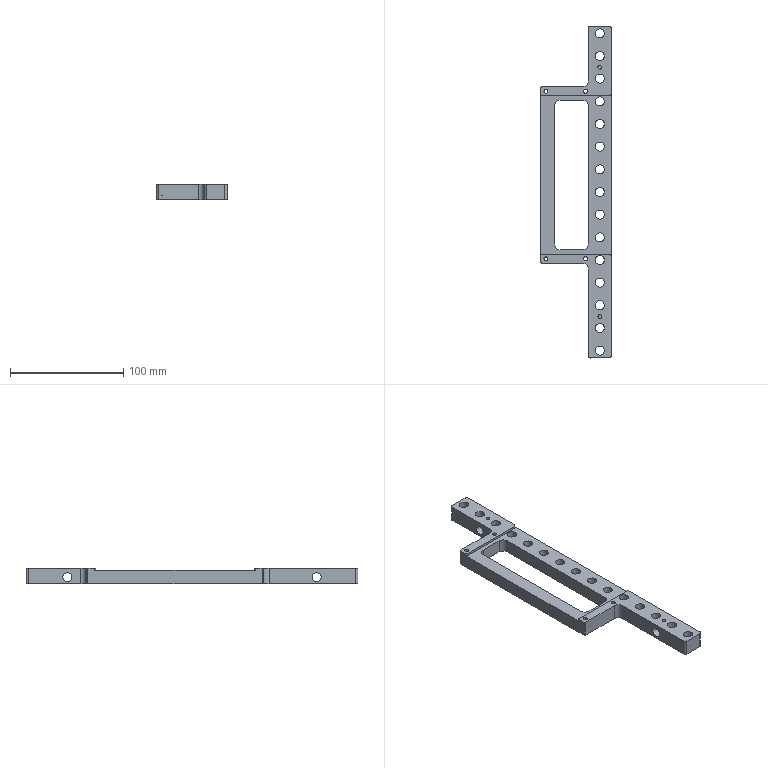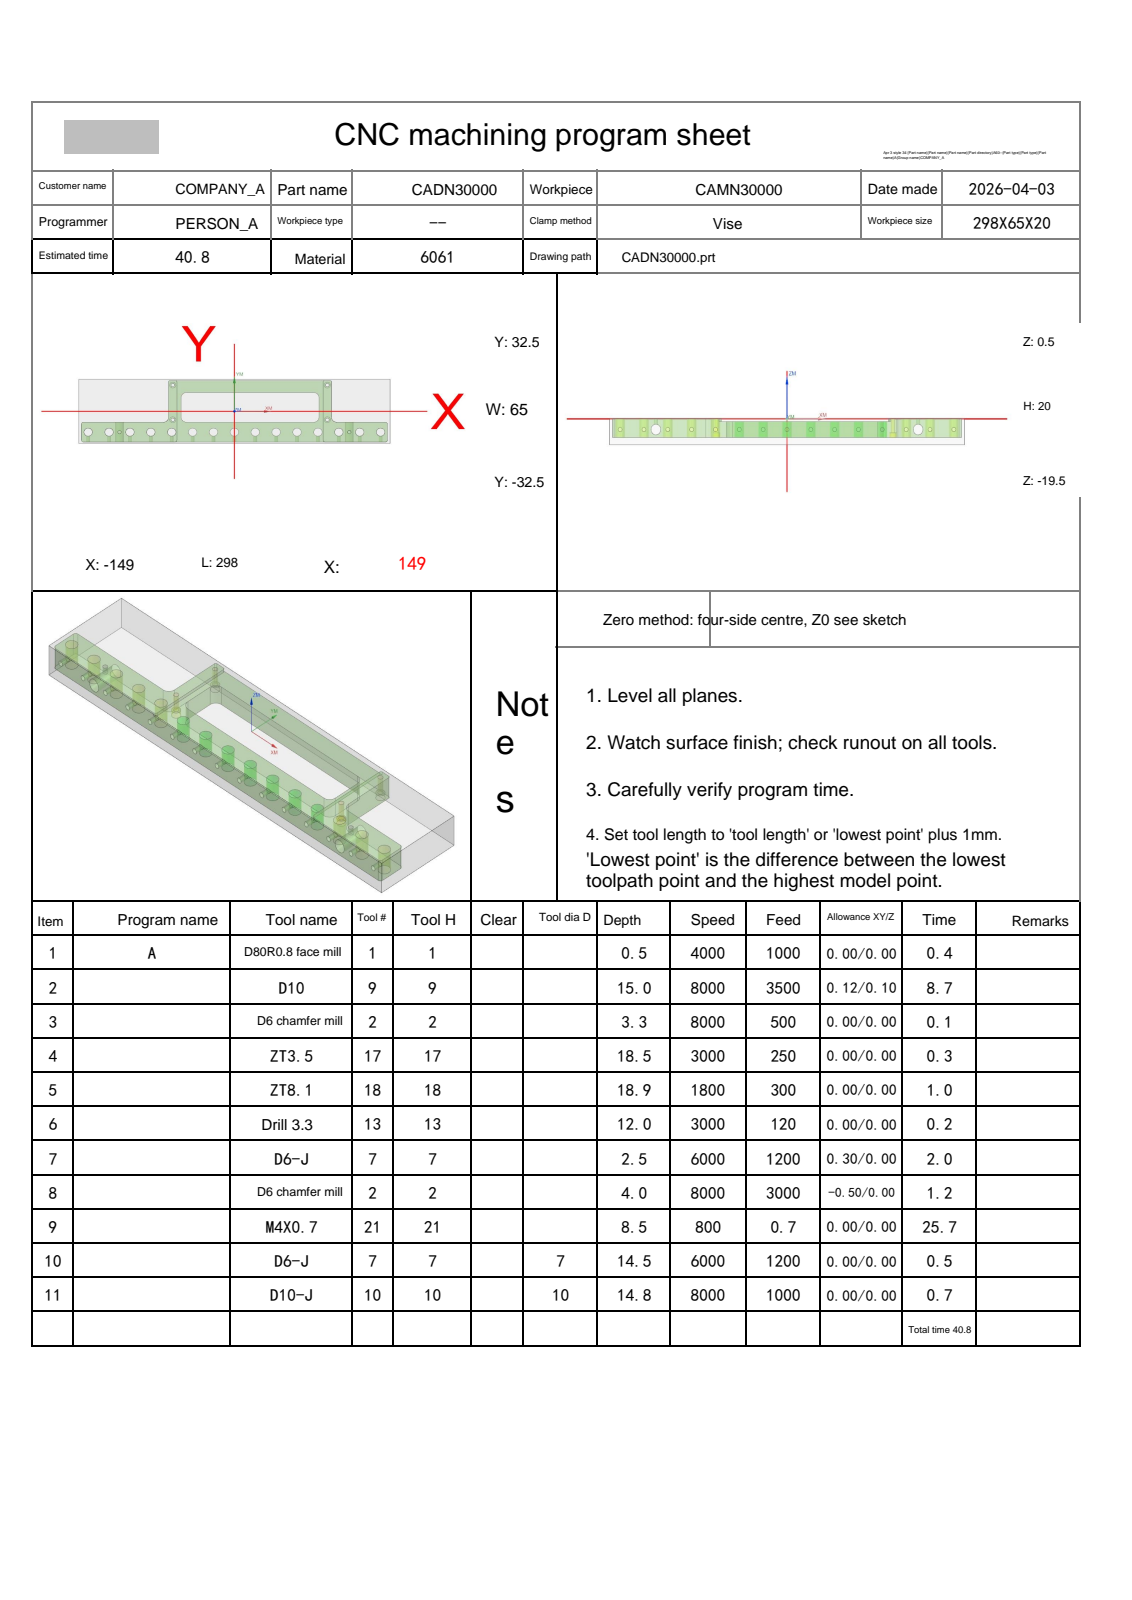NC program | NX | posted by the shop | part box 62 x 293 x 14 mm
Lines 36 to 825 of 5964:
N2 T09 M06
(D10  D=10. R=0. H=09 ce=0.12 di=0.10)
G00 G90 G54 X88.366 Y43.445 M03 S8000
G43 H09 Z20.
M08
Z-12.5
G01 X88.382 Y43.346 Z-13.125 F3500.
X88.398 Y43.248 Z-13.372
X88.414 Y43.149 Z-13.554
X88.43 Y43.05 Z-13.7
X88.446 Y42.951 Z-13.823
X88.462 Y42.853 Z-13.928
X88.477 Y42.754 Z-14.02
X88.493 Y42.655 Z-14.1
X88.509 Y42.557 Z-14.17
X88.525 Y42.458 Z-14.232
X88.541 Y42.359 Z-14.286
X88.557 Y42.26 Z-14.333
X88.573 Y42.162 Z-14.374
X88.589 Y42.063 Z-14.408
X88.605 Y41.964 Z-14.436
X88.621 Y41.866 Z-14.46
X88.637 Y41.767 Z-14.477
X88.653 Y41.668 Z-14.49
X88.669 Y41.569 Z-14.497
X88.685 Y41.471 Z-14.5
X89.019 Y39.395
G03 X89.346 Y39.001 I.503 J.084
X93.178 Y38.428 I3.876 J12.834
X101.853 Y38.295 I8.675 J282.345
X103.591 Y38.3 I0.0 J282.478
G01 X147.341 Y38.279
G02 X153.274 Y34.249 I-.2 J-6.677
X154.598 Y28.401 I-14.951 J-6.46
X154.816 Y19.492 I-182.174 J-8.909
X154.799 Y16.995 I-182.392 J0.0
G01 X154.774 Y-30.916
G02 X150.636 Y-36.838 I-6.704 J.279
X144.785 Y-38.108 I-6.434 J15.52
X136.71 Y-38.306 I-8.075 J164.923
X135.059 Y-38.297 I0.0 J165.121
G01 X-147.297 Y-38.281
G02 X-153.302 Y-34.188 I.172 J6.703
X-154.592 Y-28.479 I14.987 J6.387
X-154.808 Y-20.334 I153.312 J8.145
X-154.797 Y-18.544 I153.528 J0.0
G01 X-154.781 Y30.807
G02 X-150.823 Y36.737 I6.655 J-.155
X-145.06 Y38.085 I6.436 J-14.522
X-136.504 Y38.313 I8.556 J-160.427
X-134.284 Y38.298 I0.0 J-160.655
G01 X86.835 Y38.28
G03 X95.108 Y37.694 I15.608 J161.802
X104.71 Y37.6 I10.76 J603.908
G01 X145.579 Y37.575
G02 X152.002 Y33.432 I-.437 J-7.727
X153.764 Y27.207 I-14.23 J-7.39
X154.1 Y18.985 I-100.433 J-8.222
X154.092 Y17.697 I-100.769 J0.0
G01 X154.082 Y-28.92
G02 X149.838 Y-35.56 I-7.748 J.276
X143.669 Y-37.269 I-7.335 J14.483
X135.419 Y-37.6 I-8.25 J102.539
X134.088 Y-37.592 I0.0 J102.871
G01 X-145.579 Y-37.574
G02 X-152.028 Y-33.382 I.448 J7.745
X-153.755 Y-27.288 I14.212 J7.317
X-154.109 Y-18.528 I108.053 J8.761
X-154.094 Y-16.728 I108.408 J0.0
G01 X-154.074 Y29.079
G02 X-149.934 Y35.499 I7.732 J-.442
X-143.711 Y37.263 I7.389 J-14.205
X-135.007 Y37.608 I8.704 J-109.463
X-133.22 Y37.594 I0.0 J-109.809
G01 X85.239 Y37.58
X94.165 Y37.052
G03 X105.254 Y36.9 I11.089 J403.419
G01 X105.971
X143.761 Y36.876
G02 X151.325 Y31.864 I-.379 J-8.786
X153.058 Y25.265 I-16.654 J-7.9
X153.403 Y16.333 I-115.465 J-8.932
X153.392 Y14.774 I-115.81 J0.0
G01 X153.374 Y-27.286
G02 X149.06 Y-34.446 I-8.646 J.33
X147.589 Y-35.415 I-7.188 J9.308
X142.704 Y-36.512 I-6.118 J15.825
X133.383 Y-36.901 I-9.321 J111.513
X131.796 Y-36.889 I0.0 J111.902
G01 X120.456 Y-36.934
X-143.784 Y-36.911
G02 X-151.347 Y-31.833 I.451 J8.842
X-153.091 Y-24.951 I17.19 J8.019
X-153.407 Y-15.747 I133.706 J9.204
X-153.395 Y-13.899 I134.023 J0.0
G01 X-153.376 Y27.251
G02 X-148.452 Y34.777 I8.767 J-.362
X-141.728 Y36.561 I7.972 J-16.484
X-132.791 Y36.903 I8.937 J-116.735
X-131.237 Y36.892 I0.0 J-117.076
G01 X84.353 Y36.897
G03 X95.942 Y36.315 I40.76 J695.754
X108.127 Y36.2 I12.186 J649.067
G01 X108.771 Y36.201
X142.011 Y36.178
G02 X150.616 Y30.523 I-.151 J-9.604
X152.349 Y23.626 I-18.426 J-8.297
X152.71 Y13.834 I-132.729 J-9.792
X152.694 Y11.805 I-133.09 J0.0
G01 X152.678 Y-25.494
G02 X151.497 Y-30.094 I-10.288 J.19
G01 X151.441 Y-30.584
X150.915 Y-32.089
X150.067 Y-33.439
X148.939 Y-34.567
X147.589 Y-35.415
X146.084 Y-35.941
X144.499 Y-36.12
G03 X140.656 Y-36.111 I-3.843 J-851.591
X127.053 Y-36.22 I0.0 J-851.599
G01 X-141.947 Y-36.214
G03 X-144.09 Y-36.115 I-2.143 J-23.31
X-144.551 Y-36.12 I0.0 J-23.409
G02 X-149.503 Y-34.065 I.184 J7.44
X-151.481 Y-30.398 I5.506 J5.336
X-152.651 Y-18.3 I61.95 J12.098
G01 Y-18.008
X-152.698 Y-6.669
X-152.676 Y25.521
G02 X-147.023 Y34.115 I9.603 J-.161
X-140.126 Y35.849 I8.299 J-18.429
X-130.543 Y36.206 I9.583 J-128.416
X-128.726 Y36.193 I0.0 J-128.773
G01 X83.203 Y36.19
G03 X89.056 Y36.095 I5.853 J180.683
X92.056 Y36.12 I0.0 J180.778
G01 X95.389 Y35.757
G03 X105.774 Y35.49 I10.384 J201.862
X108.004 Y35.502 I0.0 J202.129
G01 X140.401 Y35.479
X140.483
G02 X149.893 Y29.319 I0.0 J-10.267
X151.663 Y21.93 I-20.181 J-8.74
X152.006 Y11.971 I-144.341 J-9.96
X151.993 Y10.039 I-144.684 J0.0
G01 X151.974 Y-23.971
G02 X151.62 Y-26.711 I-15.929 J.665
X151.642 Y-27.66 I-20.474 J-.95
X151.494 Y-30.114 I-20.497 J0.0
G03 X151.642 Y-27.66 I-20.349 J2.454
X151.62 Y-26.711 I-20.497 J0.0
G01 X151.6 Y-12.748
G02 X151.415 Y-3.423 I235.684 J9.325
X151.438 Y-.139 I235.869 J0.0
G03 X151.462 Y4.984 I-546.305 J5.122
X151.294 Y18.53 I-546.329 J0.0
X150.167 Y26.549 I-32.804 J-.521
X146.046 Y32.653 I-10.914 J-2.926
X140.146 Y34.657 I-6.784 J-10.285
X132.863 Y34.949 I-7.283 J-90.673
X131.335 Y34.936 I0.0 J-90.965
G01 X102.307 Y34.973
X101.985
G02 X95.085 Y35.29 I0.0 J75.218
G03 X92.93 Y36.05 I-3.605 J-6.789
G02 X95.408 Y35.119 I-1.66 J-8.189
G03 X99.93 Y34.419 I4.81 J16.098
X110.881 Y34.22 I10.952 J302.329
X114.371 Y34.241 I0.0 J302.527
G01 X134.521 Y34.207
G02 X135.037 Y34.211 I.516 J-33.098
X141.204 Y33.631 I0.0 J-33.102
X148.834 Y27.019 I-2.414 J-10.494
X150.438 Y19.518 I-22.691 J-8.776
X150.751 Y8.948 I-178.642 J-10.57
X150.735 Y6.575 I-178.954 J0.0
G03 X150.715 Y1.57 I622.281 J-5.004
X150.817 Y-9.709 I622.301 J0.0
G01 X151.441 Y-11.416
X151.62 Y-13.001
X151.441 Y-11.416
G02 X150.638 Y-9.193 I113.202 J42.201
X150.219 Y-4.29 I28.533 J4.903
X150.222 Y-3.904 I28.951 J0.0
G01 X150.114 Y13.934
Y14.014
G03 X149.36 Y22.851 I-52.142 J0.0
X146.54 Y29.26 I-14.062 J-2.361
X139.925 Y33.001 I-8.623 J-7.531
X132.902 Y33.633 I-7.023 J-38.658
G01 X132.683
X124.283 Y33.68
X104.973 Y33.716
G02 X104.369 Y33.713 I-.604 J51.363
X97.249 Y34.209 I0.0 J51.367
X96.075 Y34.556 I.273 J3.085
G01 X95.045 Y35.296
G03 X96.608 Y34.192 I15.019 J19.605
X100.851 Y33.274 I4.843 J12.127
X110.41 Y32.967 I9.559 J148.731
X112.555 Y32.983 I0.0 J149.038
G02 X118.974 Y33.004 I6.419 J-970.298
X133.331 Y32.898 I0.0 J-970.319
X140.12 Y32.046 I-.082 J-28.13
X147.592 Y25.181 I-3.085 J-10.857
X149.192 Y17.397 I-24.032 J-8.997
X149.491 Y6.608 I-195.087 J-10.789
X149.476 Y4.197 I-195.386 J0.0
G03 X149.457 Y1.765 I161.418 J-2.432
X149.674 Y-6.599 I161.436 J0.0
X149.978 Y-8.456 I6.431 J.1
G01 X150.849 Y-9.805
X149.832 Y-8.234
G02 X149.113 Y-4.484 I10.992 J4.053
X148.898 Y4.66 I194.486 J9.144
X148.908 Y6.663 I194.701 J0.0
G03 X148.918 Y8.24 I-122.885 J1.576
X148.514 Y18.202 I-122.895 J0.0
X146.65 Y25.415 I-20.899 J-1.553
X139.073 Y31.428 I-10.294 J-5.19
X131.515 Y32.335 I-7.651 J-31.802
X117.611 Y32.443 I-13.904 J-894.391
X111.855 Y32.425 I0.0 J-894.499
G02 X110.047 Y32.411 I-1.808 J119.155
X100.806 Y32.77 I0.0 J119.169
X96.864 Y33.717 I.705 J11.616
G01 X96.105 Y34.522
G03 X97.606 Y33.177 I4.301 J3.287
X102.234 Y32.076 I5.428 J12.533
X111.984 Y31.711 I9.75 J130.033
X113.888 Y31.724 I0.0 J130.398
G02 X118.722 Y31.743 I4.835 J-621.9
X131.51 Y31.612 I0.0 J-621.919
X138.767 Y30.588 I-.253 J-28.031
X146.42 Y23.228 I-3.501 J-11.299
X147.955 Y15.21 I-26.155 J-9.164
X148.243 Y3.184 I-251.31 J-12.026
X148.237 Y1.51 I-251.597 J0.0
G03 X148.231 Y.722 I51.384 J-.788
X148.671 Y-5.984 I51.39 J0.0
X149.155 Y-7.649 I5.264 J.628
G01 X149.996 Y-8.491
G02 X148.846 Y-7.204 I3.733 J4.496
X147.927 Y-3.139 I10.836 J4.586
X147.624 Y6.59 I156.211 J9.729
X147.629 Y7.812 I156.514 J0.0
G03 X147.632 Y8.505 I-76.835 J.694
X147.025 Y18.146 I-76.838 J0.0
X144.602 Y25.099 I-17.244 J-2.11
X137.389 Y30.105 I-10.102 J-6.854
X129.836 Y31.055 I-7.901 J-32.347
X115.29 Y31.184 I-14.545 J-815.993
X111.734 Y31.176 I0.0 J-816.123
G02 X110.666 Y31.17 I-1.068 J86.796
X101.749 Y31.629 I0.0 J86.803
X97.643 Y32.785 I1.053 J11.616
X96.907 Y33.658 I.902 J1.508
G03 X98.84 Y31.921 I3.016 J1.412
X104.269 Y30.787 I6.391 J17.048
X114.274 Y30.454 I10.005 J149.964
X116.058 Y30.465 I0.0 J150.297
G02 X119.471 Y30.483 I3.413 J-322.485
X130.533 Y30.293 I0.0 J-322.503
X137.685 Y29.076 I-.673 J-25.582
X145.234 Y21.349 I-4.145 J-11.601
X146.71 Y13.178 I-28.114 J-9.296
X147.023 Y1.232 I-328.91 J-14.604
G01 Y1.221
G03 X147.651 Y-5.269 I33.863 J0.0
X148.346 Y-7.049 I4.852 J.868
G02 X149.137 Y-7.631 I-1.71 J-3.154
G03 X148.278 Y-7.009 I-2.761 J-2.91
G02 X147.095 Y-4.269 I4.712 J3.659
X146.455 Y2.855 I39.504 J7.142
G03 X146.05 Y14.004 I-189.773 J-1.315
X144.364 Y21.557 I-24.465 J-1.494
X136.045 Y28.719 I-11.47 J-4.91
X128.016 Y29.785 I-8.372 J-32.301
X111.675 Y29.94 I-16.342 J-860.498
G01 X111.555
G02 X111.071 Y29.938 I-.485 J65.235
X102.171 Y30.548 I0.0 J65.237
X98.111 Y31.915 I1.389 J10.837
X97.57 Y32.535 I.443 J.933
G01 X97.285 Y33.017
X97.776 Y32.084
G03 X100.474 Y30.482 I4.167 J3.943
X107.281 Y29.423 I7.662 J26.845
X119.233 Y29.178 I11.952 J291.171
X121.734 Y29.188 I0.0 J291.416
G02 X122.976 Y29.197 I1.242 J-85.634
X131.937 Y28.727 I0.0 J-85.643
X138.915 Y26.392 I-1.675 J-16.599
X144.127 Y19.274 I-7.391 J-10.878
X145.483 Y10.935 I-31.496 J-9.401
G01 X145.872 Y.528
G03 X146.819 Y-5.251 I21.767 J.6
X147.512 Y-6.54 I3.225 J.903
G01 X148.36 Y-7.069
G02 X147.297 Y-6.38 I4.276 J7.761
X145.935 Y-3.318 I5.374 J4.224
X145.2 Y3.82 I39.475 J7.671
G03 X144.65 Y13.644 I-124.937 J-2.076
X142.528 Y21.148 I-20.959 J-1.872
X134.503 Y27.413 I-11.287 J-6.187
X126.616 Y28.503 I-8.482 J-32.308
X112.138 Y28.701 I-17.158 J-725.643
G01 X111.952 Y28.7
G02 X102.748 Y29.433 I0.0 J58.195
X98.529 Y31.006 I1.637 J10.831
X97.641 Y32.322 I.975 J1.616
G03 X99.338 Y30.169 I3.06 J.665
X104.602 Y28.568 I6.827 J12.992
X114.706 Y27.967 I10.105 J84.66
X115.396 Y27.969 I0.0 J85.261
G02 X116.713 Y27.973 I1.317 J-222.994
X127.905 Y27.692 I0.0 J-222.998
X135.413 Y26.139 I-1.033 J-23.912
X142.645 Y18.319 I-5.068 J-11.943
X144.161 Y10.296 I-28.53 J-9.546
G03 X144.714 Y.645 I830.765 J42.782
X145.872 Y-4.861 I18.699 J1.055
X146.818 Y-6.305 I3.644 J1.357
G01 X147.589 Y-6.585
G02 X146.428 Y-6.031 I.536 J2.62
X144.864 Y-2.877 I5.344 J4.614
X143.961 Y4.118 I35.441 J8.13
G03 X143.215 Y13.299 I-97.979 J-3.343
X140.689 Y20.597 I-18.635 J-2.364
X133.045 Y26.099 I-11.066 J-7.312
X124.745 Y27.245 I-8.833 J-33.348
X112.041 Y27.482 I-24.212 J-955.997
G02 X103.123 Y28.343 I.362 J50.403
X98.746 Y30.166 I1.862 J10.635
X98.009 Y31.039 I1.125 J1.698
G03 X97.871 Y31.629 I-3.67 J-.546
G01 X98.094 Y30.732
G03 X100.256 Y28.843 I4.068 J2.475
X106.133 Y27.263 I7.651 J16.741
X116.047 Y26.716 I10.002 J91.146
G01 X116.507 Y26.717
G02 X127.227 Y26.341 I0.0 J-153.093
X134.667 Y24.506 I-1.388 J-21.629
X141.382 Y16.783 I-5.915 J-11.924
X142.903 Y8.971 I-29.365 J-9.77
G03 X143.594 Y.576 I240.014 J15.551
X145.04 Y-4.796 I16.033 J1.434
X145.972 Y-6.016 I3.29 J1.547
G01 X146.843 Y-6.324
G02 X145.634 Y-5.82 I.857 J3.754
X143.891 Y-2.823 I4.609 J4.687
X142.745 Y4.032 I30.142 J8.561
G03 X141.834 Y12.491 I-87.453 J-5.136
X138.997 Y19.743 I-17.642 J-2.721
X131.316 Y24.88 I-11.053 J-8.216
X123.079 Y25.984 I-8.918 J-35.257
G01 X111.682 Y26.287
G02 X103.065 Y27.349 I.868 J42.508
X98.814 Y29.391 I2.175 J9.973
X98.081 Y30.361 I1.697 J2.045
G01 X98.014 Y30.988
Y30.959
G03 X99.096 Y28.802 I2.691 J0.0
X103.573 Y26.684 I6.783 J8.544
X112.329 Y25.598 I9.776 J42.992
G02 X123.982 Y25.208 I-19.123 J-744.989
X131.942 Y23.755 I-.999 J-28.02
X140.137 Y15.244 I-4.72 J-12.745
X141.73 Y7.159 I-32.559 J-10.614
G03 X142.715 Y-.663 I77.16 J5.741
X144.483 Y-5.136 I11.409 J1.925
X145.455 Y-5.988 I1.877 J1.162
G01 X146.084 Y-6.059
X146.011 Y-6.06
G02 X144.252 Y-5.149 I0.0 J2.153
X142.364 Y-.999 I8.217 J6.244
X141.232 Y6.584 I57.767 J12.494
G03 X139.701 Y14.399 I-35.945 J-2.987
X130.284 Y23.469 I-13.123 J-4.201
X122.067 Y24.701 I-9.157 J-33.072
G02 X110.6 Y25.158 I19.419 J630.622
X102.53 Y26.517 I1.478 J33.436
X98.725 Y28.725 I2.577 J8.822
X98.12 Y29.687 I1.583 J1.667
G01 X98.083 Y30.347
G03 X98.168 Y29.364 I14.767 J.79
X100.134 Y27.166 I4.262 J1.835
X105.962 Y25.101 I8.197 J13.87
X115.37 Y24.252 I10.709 J66.197
G02 X125.068 Y23.707 I-1.974 J-121.495
X132.549 Y21.531 I-1.839 J-20.268
X138.866 Y13.836 I-6.928 J-12.128
X140.484 Y6.465 I-33.385 J-11.191
G03 X141.701 Y-.842 I61.107 J6.421
X143.669 Y-5.099 I10.717 J2.371
X144.654 Y-5.897 I2.035 J1.506
G01 X145.419 Y-5.984
X145.369
G02 X144.155 Y-5.706 I0.0 J2.793
X142.021 Y-2.925 I3.608 J4.978
X140.39 Y3.382 I23.343 J9.4
G03 X139.048 Y10.999 I-81.989 J-10.517
X135.378 Y18.232 I-16.077 J-3.61
X127.564 Y22.542 I-10.936 J-10.589
X119.094 Y23.533 I-9.544 J-44.899
G02 X108.374 Y24.217 I3.44 J138.21
X101.314 Y26.045 I2.196 J23.024
X98.271 Y28.572 I2.654 J6.293
X98.096 Y29.366 I1.715 J.795
X98.12 Y29.667 I1.891 J0.0
G03 X98.096 Y29.303 I2.804 J-.364
X99.032 Y27.201 I2.828 J0.0
X103.562 Y24.639 I7.36 J7.726
X112.106 Y23.213 I10.481 J36.501
G02 X122.267 Y22.594 I-29.996 J-576.291
X130.074 Y20.783 I-1.629 J-24.748
X137.528 Y12.678 I-5.848 J-12.858
X139.253 Y5.832 I-33.62 J-12.112
G03 X140.759 Y-1.21 I50.777 J7.178
X142.954 Y-5.21 I9.762 J2.755
X143.952 Y-5.88 I1.67 J1.408
G01 X144.641 Y-5.896
G02 X144.423 Y-5.902 I-.217 J3.695
X143.625 Y-5.815 I0.0 J3.701
X141.476 Y-3.704 I2.251 J4.44
X139.496 Y1.797 I16.145 J8.919
G03 X137.981 Y9.094 I-243.44 J-46.732
X134.67 Y16.21 I-17.877 J-3.991
X126.887 Y21.078 I-11.38 J-9.539
X118.445 Y22.269 I-9.974 J-40.191
G02 X108.056 Y23.13 I4.617 J118.839
X101.213 Y25.139 I2.655 J21.704
X98.259 Y27.766 I2.949 J6.29
X98.097 Y28.541 I1.773 J.775
X98.12 Y28.841 I1.935 J0.0
G03 X98.1 Y28.491 I3.029 J-.35
X99.101 Y26.232 I3.05 J0.0
X103.703 Y23.559 I7.742 J8.029
X112.369 Y21.996 I11.043 J36.416
G02 X121.563 Y21.274 I-22.661 J-347.552
X129.307 Y19.212 I-1.996 J-23.071
X136.307 Y11.304 I-6.669 J-12.954
X138.166 Y4.633 I-38.729 J-14.393
G03 X140.063 Y-2.116 I35.832 J6.426
X142.566 Y-5.597 I7.696 J2.895
X143.142 Y-5.88 I1.12 J1.55
G01 X143.912
G02 X143.551 Y-5.904 I-.361 J2.767
X142.626 Y-5.746 I0.0 J2.791
X140.204 Y-3.204 I2.978 J5.262
X138.057 Y2.802 I20.622 J10.761
G03 X136.141 Y9.891 I-66.926 J-14.279
X130.826 Y17.313 I-14.562 J-4.815
X123.194 Y20.346 I-10.488 J-15.271
X114.484 Y21.269 I-13.237 J-83.368
G02 X105. Y22.671 I2.705 J51.082
X99.567 Y25.3 I3.252 J13.648
X98.12 Y27.26 I2.652 J3.472
G01 Y28.03
G03 X98.096 Y27.639 I3.18 J-.391
X99.091 Y25.319 I3.204 J0.0
X103.667 Y22.529 I7.998 J7.97
X112.105 Y20.823 I11.45 J34.92
G02 X121.288 Y19.889 I-17.64 J-219.055
X128.9 Y17.422 I-2.496 J-20.675
X135.118 Y9.955 I-7.96 J-12.95
X137.354 Y2.696 I-53.184 J-20.355
G03 X139.69 Y-3.371 I23.122 J5.421
X142.129 Y-5.854 I5.511 J2.974
G01 X143.098 Y-5.88
G02 X142.707 Y-5.905 I-.391 J3.107
X141.735 Y-5.75 I0.0 J3.132
X139.219 Y-3.251 I2.986 J5.523
X136.92 Y2.4 I20.319 J11.557
G03 X134.695 Y9.276 I-62.081 J-16.289
X124.462 Y18.463 I-14.265 J-5.596
X116.12 Y19.866 I-11.423 J-42.436
G02 X106.476 Y21.207 I5.236 J72.983
X100.297 Y23.765 I3.498 J17.193
X98.129 Y26.292 I3.137 J4.885
G01 X98.12 Y27.189
G03 X98.095 Y26.77 I3.546 J-.418
X98.325 Y25.51 I3.571 J0.0
X101.3 Y22.599 I6.329 J3.492
X108.299 Y20.211 I10.578 J19.547
X117.695 Y18.985 I21.976 J131.86
G02 X125.453 Y17.207 I-2.814 J-30.091
X133.761 Y9.095 I-5.827 J-14.276
X136.254 Y2.161 I-53.513 J-23.159
G03 X138.821 Y-3.607 I22.021 J6.344
X141.217 Y-5.859 I5.333 J3.272
G01 X142.234 Y-5.88
G02 X141.814 Y-5.905 I-.42 J3.542
X140.825 Y-5.765 I0.0 J3.567
X138.257 Y-3.377 I2.856 J5.646
X135.722 Y2.177 I20.576 J12.747
G03 X133.091 Y8.962 I-50.585 J-15.708
X123.027 Y17.252 I-14.225 J-7.015
X115.534 Y18.641 I-11.948 J-43.564
G02 X106.22 Y20.168 I6.572 J69.279
X100.099 Y22.926 I3.826 J16.66
X98.129 Y25.352 I3.333 J4.72
G01 X98.12 Y26.246
G03 X98.095 Y25.827 I3.524 J-.42
X98.37 Y24.456 I3.549 J0.0
X101.443 Y21.496 I6.68 J3.859
X108.432 Y19.041 I11.052 J20.288
X117.305 Y17.688 I28.911 J159.847
G02 X125.103 Y15.533 I-3.293 J-27.094
X132.585 Y7.92 I-7.15 J-14.51
X135.387 Y1.062 I-70.326 J-32.738
G03 X138.282 Y-4.272 I18.192 J6.42
X140.293 Y-5.872 I4.215 J3.235
G01 X141.254 Y-5.88
G02 X140.834 Y-5.905 I-.421 J3.608
X139.826 Y-5.762 I0.0 J3.633
X137.112 Y-3.281 I3.019 J6.028
X134.279 Y2.502 I24.682 J15.676
G03 X131.115 Y9.141 I-34.948 J-12.579
X121.698 Y16.035 I-13.843 J-9.031
X114.224 Y17.533 I-13.663 J-48.791
G02 X105.157 Y19.38 I6.48 J54.984
X99.603 Y22.348 I4.19 J14.52
X98.12 Y24.438 I3.107 J3.776
G01 Y25.278
G03 X98.095 Y24.858 I3.562 J-.42
X98.376 Y23.468 I3.587 J0.0
X101.533 Y20.408 I6.907 J3.968
X108.759 Y17.817 I11.722 J21.317
X117.264 Y16.317 I59.575 J312.943
G02 X124.985 Y13.682 I-3.835 J-23.867
X131.601 Y6.488 I-9.036 J-14.949
X134.582 Y.013 I-121.644 J-59.937
G03 X137.692 Y-4.777 I15.226 J6.479
X139.326 Y-5.88 I3.046 J2.752
G01 X140.306
G02 X139.849 Y-5.901 I-.457 J4.996
X138.986 Y-5.826 I0.0 J5.016
X136.364 Y-3.765 I2.269 J5.584
X133.383 Y1.437 I20.306 J15.094
G03 X130.045 Y7.823 I-41.358 J-17.552
X120.473 Y14.815 I-14.428 J-9.703
X114.264 Y16.234 I-14.035 J-47.113
G02 X105.512 Y18.161 I9.494 J63.952
X99.741 Y21.21 I4.497 J15.498
X98.12 Y23.457 I3.188 J4.008
G01 Y24.367
G03 X98.099 Y23.927 I4.573 J-.441
X98.241 Y22.792 I4.594 J0.0
X100.807 Y19.837 I6.228 J2.817
X107.451 Y16.978 I11.501 J17.576
X115.921 Y15.198 I35.314 J147.021
G02 X123.628 Y12.528 I-4.647 J-25.868
X130.362 Y5.627 I-9.324 J-15.836
X133.636 Y-.624 I-152.75 J-83.978
G03 X136.891 Y-5.04 I13.962 J6.885
X138.263 Y-5.88 I2.628 J2.751
G01 X139.313
G02 X138.863 Y-5.894 I-.451 J7.062
X137.942 Y-5.834 I0.0 J7.076
X135.202 Y-3.744 I2.301 J5.854
X131.973 Y1.47 I23.435 J18.121
G03 X128.004 Y7.857 I-31.953 J-15.433
X118.931 Y13.73 I-14.266 J-12.094
X111.222 Y15.545 I-21.812 J-75.339
G02 X103.054 Y18.036 I6.601 J36.287
X98.684 Y21.354 I4.451 J10.398
X98.12 Y22.448 I3.116 J2.3
G01 Y23.358
G03 X98.096 Y22.91 I4.108 J-.448
X98.3 Y21.626 I4.132 J0.0
X101.071 Y18.599 I6.7 J3.351
X108.041 Y15.653 I12.431 J19.699
X116.018 Y13.771 I127.377 J521.916
G02 X123.891 Y10.39 I-5.184 J-22.933
X129.822 Y3.699 I-12.791 J-17.311
G03 X133.244 Y-2.09 I154.932 J87.676
X136.474 Y-5.558 I10.038 J6.113
X137.161 Y-5.88 I1.724 J2.778
G01 X138.211
G02 X137.735 Y-5.898 I-.476 J6.203
X136.824 Y-5.831 I0.0 J6.222
X134.112 Y-3.858 I2.323 J6.041
X131.074 Y.519 I21.928 J18.464
G03 X126.948 Y6.625 I-36.698 J-20.351
X117.658 Y12.597 I-15.075 J-13.241
X109.827 Y14.633 I-31.473 J-104.937
G02 X102.189 Y17.398 I6.805 J30.726
X98.461 Y20.664 I4.516 J8.917
X98.12 Y21.423 I4.091 J2.293
G01 Y22.333
G03 X98.095 Y21.882 I4.112 J-.451
X98.306 Y20.58 I4.136 J0.0
X101.102 Y17.508 I6.861 J3.436
X107.983 Y14.484 I13.047 J20.348
G02 X115.969 Y12.337 I-234.723 J-888.76
X124.623 Y7.7 I-5.859 J-21.329
X129.478 Y1.665 I-19.975 J-21.038
G03 X133.182 Y-3.664 I39.914 J23.795
X135.946 Y-5.869 I6.171 J4.899
G01 X137.134 Y-5.88
G02 X136.636 Y-5.898 I-.497 J7.046
X135.677 Y-5.832 I0.0 J7.064
X132.803 Y-3.785 I2.438 J6.461
X129.192 Y1.109 I30.716 J26.447
G03 X123.985 Y7.325 I-25.063 J-15.706
X115.413 Y11.825 I-15.069 J-18.289
G01 X107.625 Y14.042
G02 X100.827 Y17.184 I6.441 J22.859
X98.14 Y20.282 I4.117 J6.285
G01 X98.12 Y21.297
G03 X98.096 Y20.847 I4.215 J-.449
X98.299 Y19.552 I4.239 J0.0
X101.132 Y16.403 I7.01 J3.458
X108.137 Y13.231 I13.961 J21.513
G02 X115.939 Y10.856 I-57.678 J-203.43
X127.159 Y2.583 I-7.357 J-21.722
G03 X131.228 Y-2.898 I160.351 J114.799
X134.608 Y-5.822 I8.554 J6.473
X135.52 Y-5.904 I.911 J5.011
X136.011 Y-5.88 I0.0 J5.093
G02 X135.529 Y-5.892 I-.482 J10.051
X134.495 Y-5.838 I0.0 J10.062
X131.564 Y-3.851 I2.414 J6.714
X127.715 Y.913 I35.884 J32.929
G03 X121.563 Y7.204 I-22.93 J-16.273
X113.467 Y11.011 I-16.229 J-23.996
G02 X105.58 Y13.58 I35.916 J123.685
X99.871 Y16.882 I6.273 J17.428
X98.12 Y19.324 I3.715 J4.514
G01 Y20.304
G03 X98.098 Y19.835 I4.946 J-.469
X98.244 Y18.637 I4.969 J0.0
X100.827 Y15.529 I6.716 J2.954
X107.463 Y12.236 I14.102 J20.082
G02 X115.111 Y9.652 I-83.62 J-260.121
X126.235 Y1.51 I-8.892 J-23.819
G03 X130.541 Y-3.66 I73.916 J57.196
X133.525 Y-5.875 I6.596 J5.768
G01 X134.82 Y-5.88
G02 X134.293 Y-5.894 I-.527 J10.053
X133.229 Y-5.838 I0.0 J10.067
X130.306 Y-3.957 I2.45 J7.021
X126.049 Y.849 I44.358 J43.576
G03 X113.516 Y9.565 I-21.289 J-17.243
G02 X105.826 Y12.296 I78.365 J232.911
X99.865 Y15.797 I6.778 J18.363
X98.12 Y18.255 I3.823 J4.563
G01 Y19.235
G03 X98.099 Y18.77 I5.269 J-.465
X98.23 Y17.603 I5.289 J0.0
X100.667 Y14.543 I6.651 J2.797
X107.088 Y11.143 I14.506 J19.629
G02 X114.584 Y8.347 I-84.386 J-237.711
X125.103 Y.732 I-10.846 J-26.053
G03 X129.592 Y-4.109 I57.581 J48.895
X132.156 Y-5.864 I6.417 J6.624
G01 X133.506 Y-5.88
G02 X133.046 Y-5.888 I-.46 J13.818
X131.916 Y-5.842 I0.0 J13.826
X128.861 Y-3.955 I2.548 J7.544
X124.347 Y.706 I63.767 J66.28
G03 X112.762 Y8.405 I-22.117 J-20.711
G02 X105.043 Y11.432 I60.174 J164.81
X99.544 Y15.008 I6.955 J16.715
X98.12 Y17.172 I3.792 J4.046
G01 Y18.152
G03 X98.095 Y17.672 I4.617 J-.48
X98.287 Y16.35 I4.642 J0.0
X100.936 Y13.204 I7.239 J3.407
X107.476 Y9.731 I16.213 J22.637
G02 X115.13 Y6.538 I-38.187 J-102.302
X124.282 Y-.342 I-14.78 J-29.186
G03 X128.793 Y-4.67 I36.361 J33.388
X130.859 Y-5.88 I4.451 J5.231
G01 X132.189
G02 X131.591 Y-5.905 I-.599 J7.198
X130.346 Y-5.797 I0.0 J7.223
X127.022 Y-3.69 I3.519 J9.228
X122.053 Y1.002 I488.449 J522.287
G03 X111.277 Y7.577 I-23.5 J-26.395
G02 X103.88 Y10.801 I32.684 J85.091
X99.112 Y14.372 I6.865 J14.135
X98.12 Y16.073 I3.87 J3.398
G01 Y17.053
G03 X98.095 Y16.573 I4.644 J-.48
X98.291 Y15.235 I4.669 J0.0
X100.919 Y12.07 I7.365 J3.441
X107.146 Y8.585 I16.946 J22.981
G02 X114.968 Y5.024 I-38.636 J-95.209
X123.551 Y-1.432 I-19.476 J-34.83
G03 X128.148 Y-5.273 I22.602 J22.377
X129.394 Y-5.88 I3.216 J5.02
G01 X130.794
G02 X130.324 Y-5.886 I-.47 J19.334
X129.054 Y-5.844 I0.0 J19.34
X125.861 Y-4.077 I2.652 J8.56
X120.492 Y.517 I243.93 J290.52
G03 X110.224 Y6.617 I-26.36 J-32.682
G02 X103.121 Y10.02 I26.775 J65.004
X98.819 Y13.624 I6.751 J12.43
X98.12 Y14.958 I3.865 J2.873
G01 Y15.938
G03 X98.095 Y15.457 I4.696 J-.482
X98.293 Y14.105 I4.72 J0.0
X101.003 Y10.834 I7.652 J3.581
X107.314 Y7.198 I18.892 J25.494
G02 X115.323 Y3.198 I-32.979 J-76.053
X122.894 Y-2.509 I-28.849 J-46.149
G03 X127.329 Y-5.69 I15.169 J16.467
G01 X127.836 Y-5.88
X129.376
G02 X128.689 Y-5.905 I-.687 J9.547
X127.312 Y-5.805 I0.0 J9.572
X123.792 Y-3.823 I3.748 J10.772
G03 X117.642 Y.945 I-126.999 J-157.46
X109.644 Y5.473 I-29.757 J-43.237
G02 X102.567 Y9.149 I25.975 J58.658
X98.612 Y12.787 I6.643 J11.19
X98.12 Y13.824 I4.236 J2.646
G01 Y14.874
G03 X98.099 Y14.377 I5.893 J-.496
X98.228 Y13.151 I5.914 J0.0
X100.649 Y9.942 I7.219 J2.928
X106.433 Y6.302 I18.166 J22.451
G02 X114.551 Y2.045 I-50.21 J-105.621
X122.009 Y-3.324 I-41.687 J-65.774
G03 X126.091 Y-5.865 I11.411 J13.784
G01 X127.789 Y-5.88
G02 X127.072 Y-5.904 I-.717 J10.738
X125.654 Y-5.81 I0.0 J10.762
X122.005 Y-3.879 I3.833 J11.657
G03 X115.198 Y.927 I-95.485 J-128.001
X106.828 Y5.479 I-51.487 J-84.71
G02 X100.504 Y9.484 I13.444 J28.224
X98.128 Y12.615 I5.046 J6.296
G01 X98.12 Y13.719
G03 X98.1 Y13.224 I6.103 J-.495
X98.222 Y12.006 I6.123 J0.0
X100.536 Y8.838 I7.244 J2.861
X106.463 Y4.945 I19.509 J23.244
G02 X115.382 Y-.087 I-49.016 J-97.304
G01 X121.763 Y-4.507
G03 X124.414 Y-5.88 I6.922 J10.115
G01 X126.164
G02 X125.386 Y-5.903 I-.777 J13.418
X123.902 Y-5.82 I0.0 J13.441
X120.27 Y-4.043 I3.719 J12.199
G03 X112.36 Y1.08 I-97.328 J-141.612
G02 X104.314 Y5.546 I476.229 J867.503
X99.239 Y9.579 I9.56 J17.238
X98.12 Y11.493 I4.374 J3.842
G01 Y12.543
G03 X98.1 Y12.048 I6.098 J-.495
X98.225 Y10.818 I6.118 J0.0
X100.546 Y7.603 I7.442 J2.93
X106.631 Y3.485 I21.42 J25.091
G02 X119.135 Y-4.118 I-70.784 J-130.495
G03 X122.531 Y-5.88 I9.082 J13.352
G01 X124.281
G02 X123.517 Y-5.899 I-.764 J15.399
X122.021 Y-5.826 I0.0 J15.418
X118.128 Y-4.021 I3.871 J13.448
G03 X105.491 Y3.512 I-139.283 J-219.303
G02 X99.892 Y7.632 I12.954 J23.466
X98.12 Y10.3 I4.817 J5.122
G01 Y11.42
G03 X98.1 Y10.893 I6.776 J-.527
X98.214 Y9.65 I6.796 J0.0
X100.499 Y6.399 I7.514 J2.851
X106.388 Y2.24 I22.16 J25.129
G02 X117.722 Y-4.554 I-295.862 J-506.444
G03 X120.532 Y-5.88 I8.042 J13.404
G01 X122.422
G02 X121.611 Y-5.897 I-.811 J18.898
X120.008 Y-5.829 I0.0 J18.915
X116.003 Y-4.077 I3.869 J14.289
X104.264 Y2.92 I284.986 J491.526
X99.268 Y7.094 I11.105 J18.369
X98.12 Y9.082 I4.687 J4.031
G01 Y10.202
G03 X98.099 Y9.675 I6.691 J-.527
X98.221 Y8.405 I6.712 J0.0
X100.5 Y5.127 I7.74 J2.95
X106.73 Y.631 I24.202 J26.971
X116.273 Y-4.967 I116.713 J188.042
X118.404 Y-5.88 I7.792 J15.238
G01 X120.434
G02 X119.507 Y-5.902 I-.927 J19.655
X117.885 Y-5.835 I0.0 J19.677